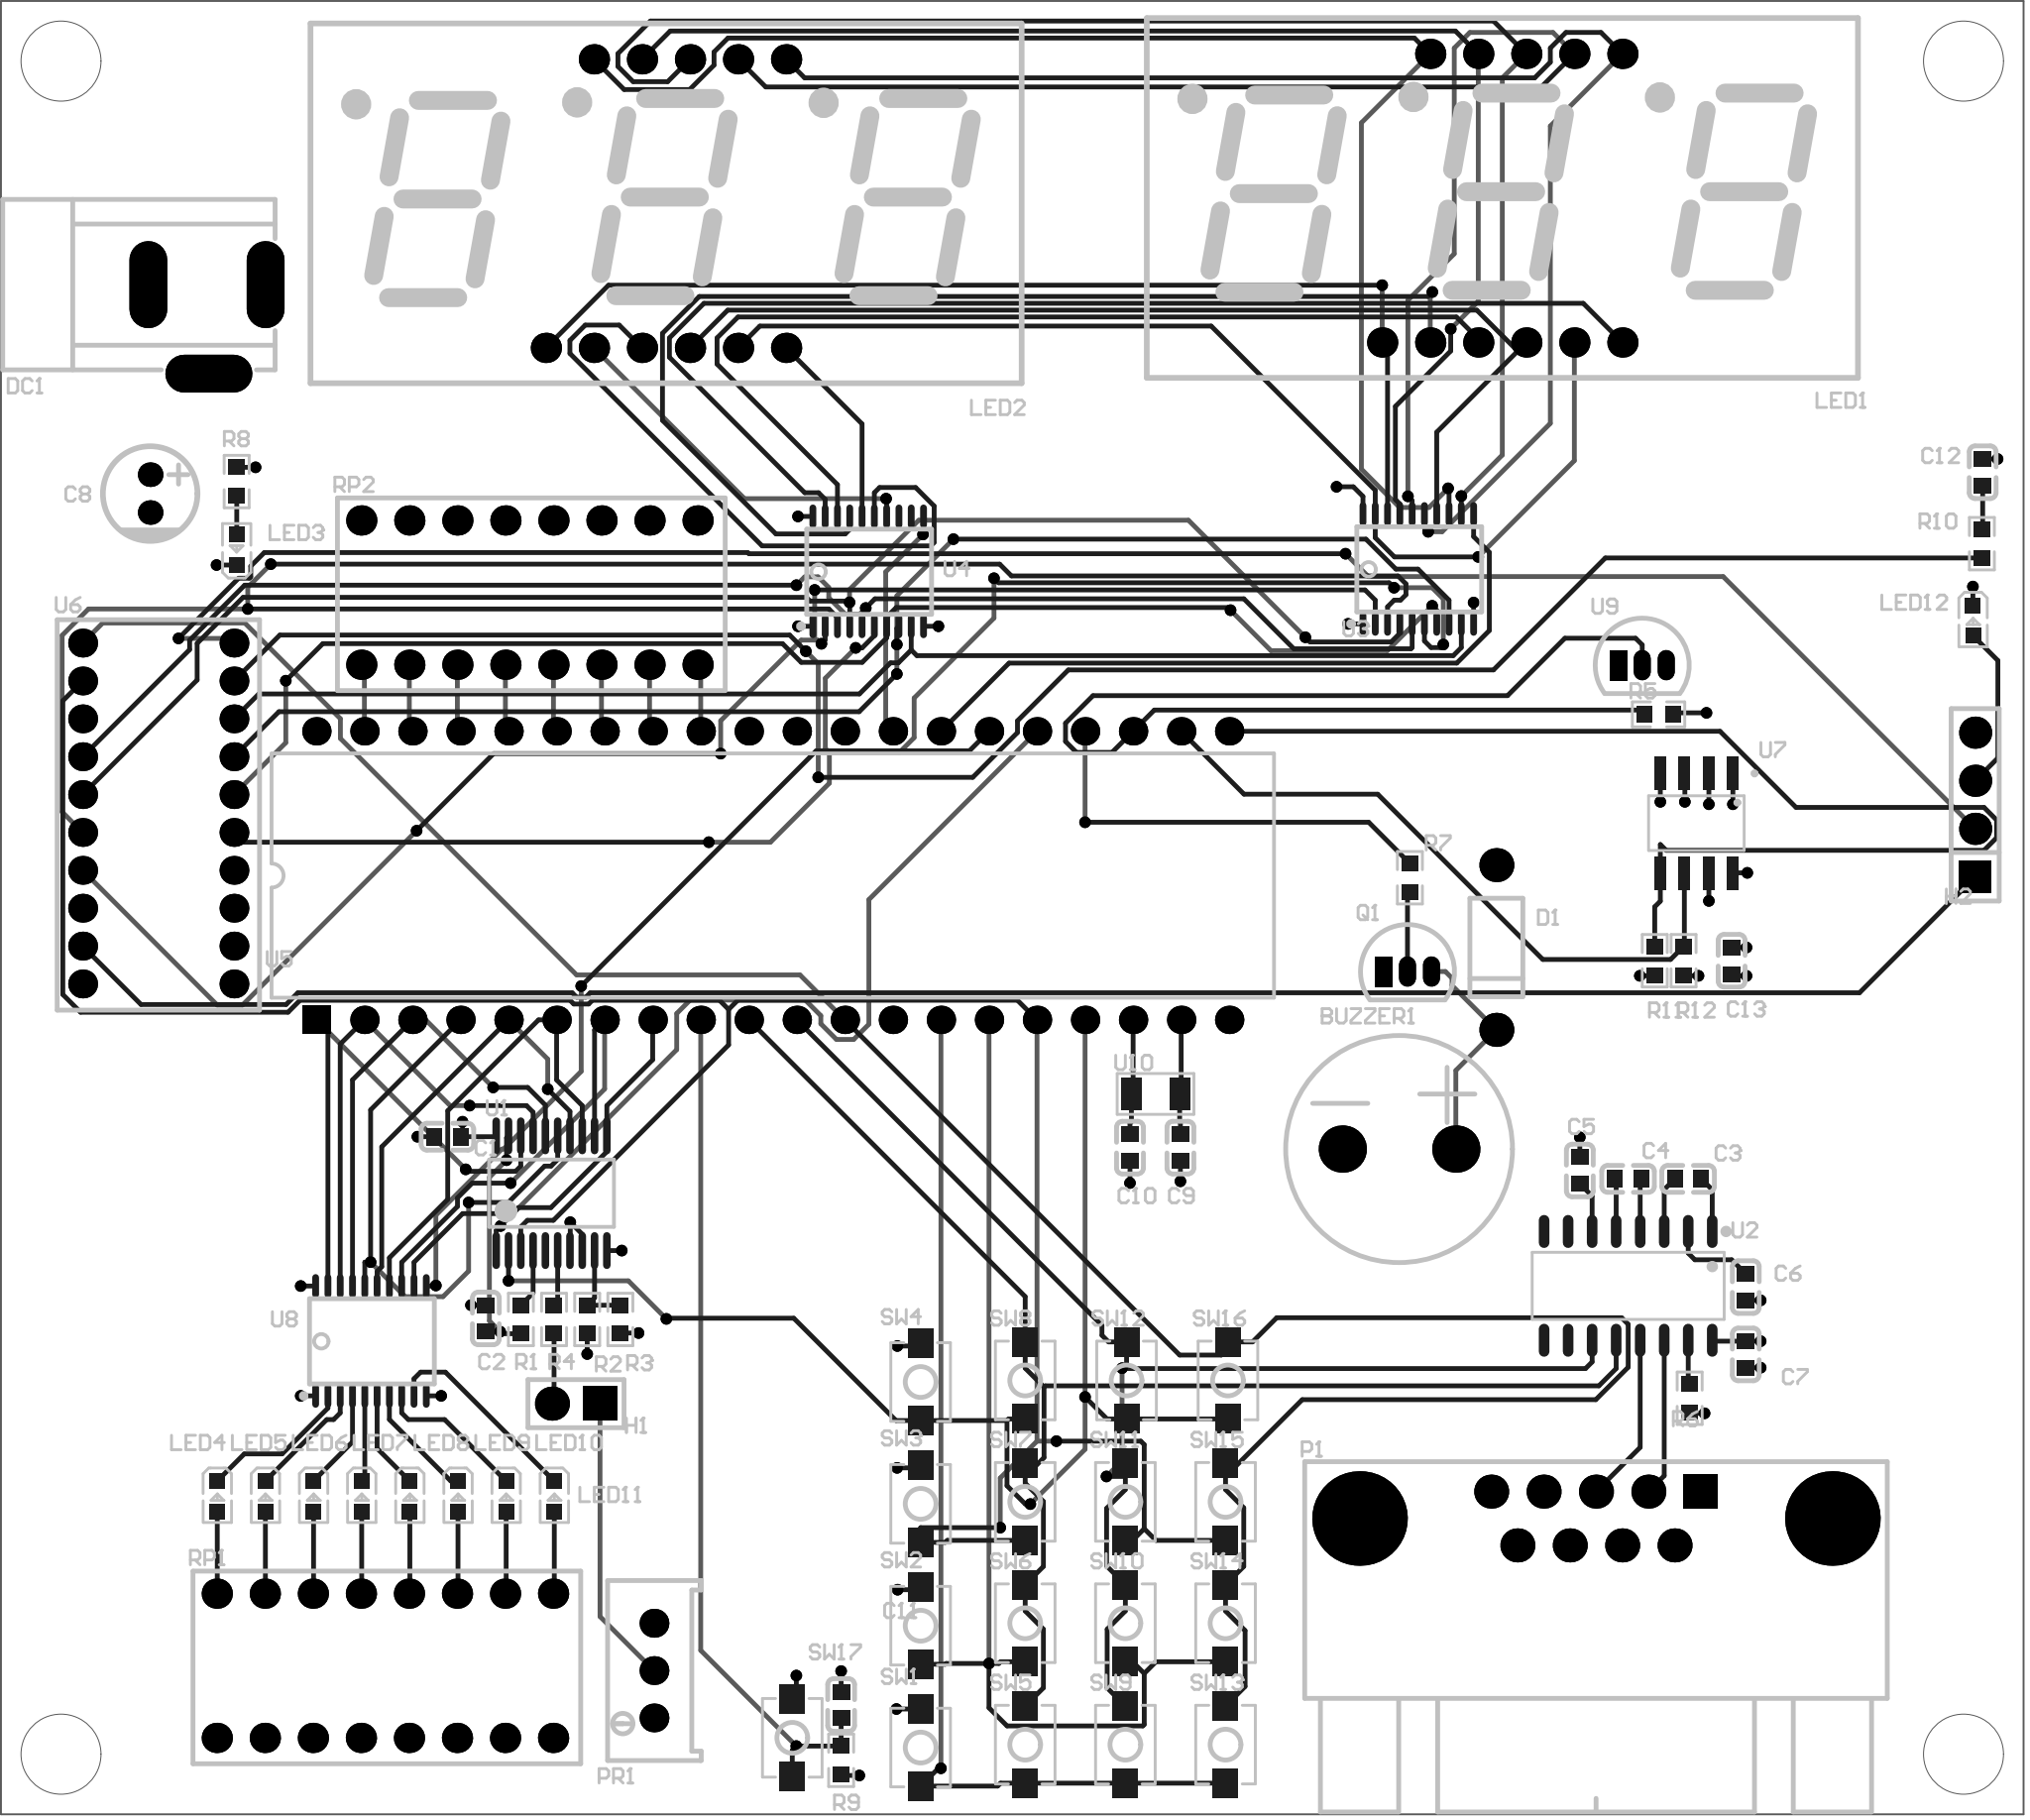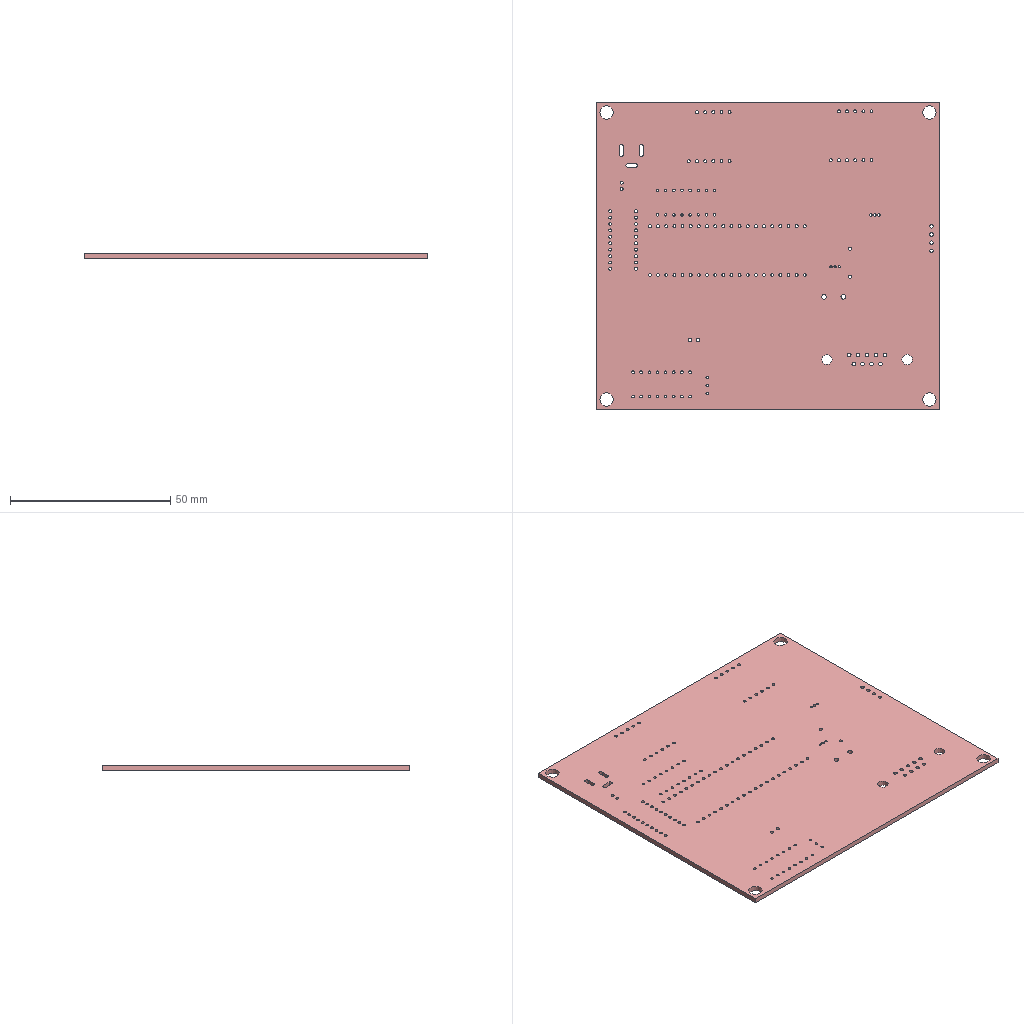Circuit board layout | Altium Designer | box 106.9 x 95.8 x 1.6 mm
Layer stack:
# Altium Designer layer stack of  (unit mm; dielectric type: 0 none, 1 core, 2 prepreg, 3 surface material)
index,name,kind,layer,copper_thickness_mm,dielectric_type,dielectric_thickness_mm,dielectric_material,dielectric_constant
0,Top Paste Mask Layer,other,,,,,,
1,Top Silkscreen Layer,other,,,,,,
2,Top Solder Mask Layer,dielectric,,,3,0,,0
3,Top Layer,copper,Top Layer,0.035,,,,
4,Dielectric1,dielectric,,,3,0.2104,7628 RC49% 8.6mil,4.4
5,Inner1,copper,Inner1,0.0152,,,,
6,Dielectric2,dielectric,,,3,1.065,1.1mm H/HOZ Copper,4.43
7,Inner2,copper,Inner2,0.0152,,,,
8,Dielectric3,dielectric,,,3,0.2104,7628 RC49% 8.6mil,4.4
9,Bottom Layer,copper,Bottom Layer,0.035,,,,
10,Bottom Solder Mask Layer,dielectric,,,3,0,,0
11,Bottom Silkscreen Layer,other,,,,,,
12,Bottom Paste Mask Layer,other,,,,,,
# drill layer pairs: low layer,high layer
drill_pair,Top Layer,Bottom Layer
Part placement:
Designator,Comment,Layer,Footprint,Center-X(mm),Center-Y(mm),Rotation
BUZZER1,buzzer,TopLayer,BUZ-TH_BD12.0-P6.00-D0.9-RD,150.118,111.331,0
C1,104,TopLayer,C0603,99.803,111.983,180
C2,104,TopLayer,C0603,101.835,102.387,90
C3,104,TopLayer,C0603,165.399,109.756,180
C4,104,TopLayer,C0603,162.224,109.756,180
C5,104,TopLayer,C0603,159.673,110.199,270
C6,104,TopLayer,C0603,168.447,104.041,90
C7,104,TopLayer,C0603,168.447,100.485,90
C8,100uF,TopLayer,CAP-TH_BD5.0-P2.00-D0.8-FD-10UF50VC110GL,84.09,145.944,270
C9,20PF,TopLayer,C0603,138.558,111.405,90
C10,20PF,TopLayer,C0603,135.891,111.405,90
C11,10uF,TopLayer,C0603,120.621,81.972,90
C12,104,TopLayer,C0603,180.972,147.072,90
C13,104,TopLayer,C0603,167.699,121.275,270
D1,,TopLayer,DO_1N4007,155.262,121.975,90
DC1,,TopLayer,DC-005_2.5,87.093,154.629,180
H1,,TopLayer,HDR-TH_2P-P2.54-V-M-1,106.602,97.886,180
H2,,TopLayer,HDR-TH_4P-P2.54-V-M,180.576,129.509,90
LED1,3631BS,TopLayer,LED-SEG-TH_11P-L37.5-W19.0-P2.54-LS15.2-BL_1,155.575,161.544,180
LED2,3631BS,TopLayer,LED-SEG-TH_11P-L37.5-W19.0-P2.54-LS15.2-BL_1,111.361,161.259,180
LED3,,TopLayer,LED_0603,88.669,142.972,90
LED4,,TopLayer,LED_0603,87.633,92.999,270
LED5,,TopLayer,LED_0603,90.179,92.999,270
LED6,,TopLayer,LED_0603,92.724,92.999,270
LED7,,TopLayer,LED_0603,95.27,92.999,270
LED8,,TopLayer,LED_0603,97.815,92.999,270
LED9,,TopLayer,LED_0603,100.361,92.999,270
LED10,,TopLayer,LED_0603,102.906,92.999,270
LED11,,TopLayer,LED_0603,105.452,92.999,270
LED12,,TopLayer,LED_0603,180.459,139.243,270
P1,DB9FL,TopLayer,DB9-TH_DB9F,160.528,91.821,0
PR1,10kΩ,TopLayer,R_3296,110.725,83.789,90
Q1,,TopLayer,S8550P_TO-92,150.563,120.705,0
R1,10K,TopLayer,R0603,103.689,102.331,90
R2,1K,TopLayer,R0603,107.195,102.331,270
R3,1K,TopLayer,R0603,108.948,102.331,90
R4,510K,TopLayer,R0603,105.442,102.331,90
R5,4.7K,TopLayer,R0603,163.836,134.284,0
R6,0,TopLayer,R0603,165.481,98.171,90
R7,2K,TopLayer,R0603,150.69,125.658,270
R8,1K,TopLayer,R0603,88.662,146.579,90
R9,10K,TopLayer,R0603,120.621,79.051,90
R10,0,TopLayer,R0603,180.93,143.299,90
R11,4.7K,TopLayer,R0603,163.635,121.275,270
R12,4.7K,TopLayer,R0603,165.159,121.275,270
RP1,,TopLayer,DIP-16_L20.3-W10.2-P2.54-LS7.6-BL,96.501,84.043,0
RP2,,TopLayer,DIP-16_L20.3-W10.2-P2.54-LS7.6-BL,104.14,140.716,0
SW1,,TopLayer,Key_SMD_3x4x2,124.823,79.725,270
SW2,,TopLayer,Key_SMD_3x4x2,124.823,86.16,270
SW3,,TopLayer,Key_SMD_3x4x2,124.823,92.594,270
SW4,,TopLayer,Key_SMD_3x4x2,124.823,99.029,270
SW5,,TopLayer,Key_SMD_3x4x2,130.352,79.88,90
SW6,,TopLayer,Key_SMD_3x4x2,130.352,86.29,90
SW7,,TopLayer,Key_SMD_3x4x2,130.352,92.7,90
SW8,,TopLayer,Key_SMD_3x4x2,130.352,99.111,90
SW9,,TopLayer,Key_SMD_3x4x2,135.647,79.88,90
SW10,,TopLayer,Key_SMD_3x4x2,135.647,86.29,90
SW11,,TopLayer,Key_SMD_3x4x2,135.647,92.7,90
SW12,,TopLayer,Key_SMD_3x4x2,135.711,99.111,90
SW13,,TopLayer,Key_SMD_3x4x2,140.943,79.88,90
SW14,,TopLayer,Key_SMD_3x4x2,140.943,86.29,90
SW15,,TopLayer,Key_SMD_3x4x2,140.943,92.7,90
SW16,,TopLayer,Key_SMD_3x4x2,141.07,99.111,90
SW17,,TopLayer,Key_SMD_3x4x2,118.037,80.239,270
U1,ADC0804CN,TopLayer,ADC0804CN,105.308,108.999,0
U2,MAX232ESE,TopLayer,MAX232ESE,162.23,104.106,180
U3,MC74HC573DW,TopLayer,MC74HC573DW,151.134,141.965,90
U4,MC74HC573DW,TopLayer,MC74HC573DW,122.051,141.838,90
U5,P89C51RC2HBP,TopLayer,P89C51RC23N_01,117.007,125.773,0
U7,AT24C02,TopLayer,SOIC-8_L5.0-W4.0-P1.27-LS6.2-TL,165.836,128.541,270
U8,MC74HC573DW,TopLayer,MC74HC573DW,95.762,101.198,90
U9,DS18B20,TopLayer,TO-92-3_L4.9-W3.7-P1.27-L,162.973,136.884,0
U10,32768/10ppm/12.5pF,TopLayer,osc-smd_l3.2-w1.5,137.242,114.241,0
U6,DAC0832LCJ,TopLayer,DAC0832LCJ,84.519,129.049,0
Pad and via stacks:
# Altium Designer via and pad stacks of  (unit mm). Each distinct definition once, with the count of objects using it.
# via: kind,start_layer,end_layer,hole_mm,diameter_mm,mode(0 simple;1 top-mid-bottom;2 full stack),diameter_per_layer,count,example_net
# pad: kind,layer,hole_mm,hole_type(0 round;1 square;2 slot),plating,top_size,top_shape(1 round;2 rect;3 octagon;9 rounded rect),mid_size,bottom_size,mode,footprint,size_per_layer,count,example
pad,Multi-Layer,1.5,0,plated,2.5x2.5,1,2.5x2.5,2.5x2.5,0,BUZ-TH_BD12.0-P6.00-D0.9-RD,,2,BUZZER1.1
pad,Multi-Layer,0.9,0,plated,1.3x1.3,1,1.3x1.3,1.3x1.3,0,CAP-TH_BD5.0-P2.00-D0.8-FD-10UF50VC110GL,,2,C8.2
pad,Multi-Layer,1,0,plated,1.8x1.8,1,1.8x1.8,1.8x1.8,0,DO_1N4007,,2,D1.1
pad,Multi-Layer,1.2,2,plated,2x4.6,1,2x4.6,2x4.6,0,DC-005_2.5,,2,DC1.1
pad,Multi-Layer,1.2,2,plated,4.6x2,1,4.6x2,4.6x2,0,DC-005_2.5,,1,DC1.3
pad,Multi-Layer,1.1,0,plated,1.8x1.8,1,1.8x1.8,1.8x1.8,0,HDR-TH_2P-P2.54-V-M-1,,1,H1.2
pad,Multi-Layer,1.1,0,plated,1.8x1.8,2,1.8x1.8,1.8x1.8,0,HDR-TH_2P-P2.54-V-M-1,,1,H1.1
pad,Multi-Layer,1.1,0,plated,1.7x1.7,2,1.7x1.7,1.7x1.7,0,HDR-TH_4P-P2.54-V-M,,1,H2.1
pad,Multi-Layer,1.1,0,plated,1.7x1.7,1,1.7x1.7,1.7x1.7,0,HDR-TH_4P-P2.54-V-M,,3,H2.2
pad,Multi-Layer,0.9,0,plated,1.6x1.6,1,1.6x1.6,1.6x1.6,0,LED-SEG-TH_11P-L37.5-W19.0-P2.54-LS15.2-BL_1,,22,LED1.4
pad,Multi-Layer,3.25,0,plated,5x5,1,5x5,5x5,0,DB9-TH_DB9F,,2,P1.10
pad,Multi-Layer,1.1,0,plated,1.8x1.8,1,1.8x1.8,1.8x1.8,0,DB9-TH_DB9F,,8,P1.6
pad,Multi-Layer,1.1,0,plated,1.8x1.8,2,1.8x1.8,1.8x1.8,0,DB9-TH_DB9F,,1,P1.1
pad,Multi-Layer,0.762,0,plated,1.524x1.524,1,1.524x1.524,1.524x1.524,0,R_3296,,3,PR1.2
pad,Multi-Layer,0.7,0,plated,0.9x1.6,1,0.9x1.6,0.9x1.6,0,S8550P_TO-92,,2,Q1.3
pad,Multi-Layer,0.7,0,plated,0.9x1.6,2,0.9x1.6,0.9x1.6,0,S8550P_TO-92,,1,Q1.1
pad,Multi-Layer,0.8,0,plated,1.6x1.6,1,1.6x1.6,1.6x1.6,0,DIP-16_L20.3-W10.2-P2.54-LS7.6-BL,,32,RP1.1
pad,Multi-Layer,0.9,2,plated,1.5x1.5,1,1.5x1.5,1.5x1.5,0,P89C51RC23N_01,,39,U5.21
pad,Multi-Layer,0.9,2,plated,1.5x1.5,2,1.5x1.5,1.5x1.5,0,P89C51RC23N_01,,1,U5.1
pad,Multi-Layer,0.8,0,plated,0.9x1.6,1,0.9x1.6,0.9x1.6,0,TO-92-3_L4.9-W3.7-P1.27-L,,2,U9.3
pad,Multi-Layer,0.8,0,plated,0.9x1.6,2,0.9x1.6,0.9x1.6,0,TO-92-3_L4.9-W3.7-P1.27-L,,1,U9.1
pad,Multi-Layer,0.9144,0,plated,1.524x1.524,1,1.524x1.524,1.524x1.524,0,DAC0832LCJ,,20,U6.1
pad,Top Layer,0,0,plated,0.8x0.9,2,0.8x0.9,0.8x0.9,0,C0603,,24,C1.2
pad,Top Layer,0,0,plated,0.8001x0.8001,2,0.8001x0.8001,0.8001x0.8001,0,LED_0603,,20,LED3.1
pad,Top Layer,0,0,plated,0.8065x0.864,2,0.8065x0.864,0.8065x0.864,0,R0603,,24,R1.2
pad,Top Layer,0,0,plated,1.53x1.36,2,1.53x1.36,1.53x1.36,0,Key_SMD_3x4x2,,34,SW1.1
pad,Top Layer,0,0,plated,0.4x1.95,1,0.4x1.95,0.4x1.95,0,ADC0804CN,,20,U1.11
pad,Top Layer,0,0,plated,0.56x1.745,1,0.56x1.745,0.56x1.745,0,MAX232ESE,,16,U2.9
pad,Top Layer,0,0,plated,1.26x0.36,1,1.26x0.36,1.26x0.36,0,MC74HC573DW,,60,U3.1
pad,Top Layer,0,0,plated,1.751x0.5887,2,1.751x0.5887,1.751x0.5887,0,SOIC-8_L5.0-W4.0-P1.27-LS6.2-TL,,8,U7.1
pad,Top Layer,0,0,plated,1.05x1.7,2,1.05x1.7,1.05x1.7,0,osc-smd_l3.2-w1.5,,2,U10.1
via,Top Layer,Bottom Layer,0.3048,0.6101,0,,57,RST
via,Top Layer,Bottom Layer,0.3048,0.61,0,,47,VCC
Design rules, without the lines most boards share:
# Altium Designer design rules of  (exported by Altium Designer, unit mm)
# columns: name | kind | enabled | priority | scope1 | scope2 | descriptor | typed fields (field=value)
creepage | 65 | enabled | 1 | All | All | Creepage Distance Constraint =(0mil) (All),(All) |
PWR | 2 | enabled | 2 | (InNet('VCC')) | All | Width Constraint (Min=10mil) (Max=100mil) (Preferred=30mil) ((InNet('VCC'))) |
copperThickness1oz_2 | 2 | enabled | 3 | All | All | Width Constraint (Min=10mil) (Max=100mil) (Preferred=10mil) (All) |